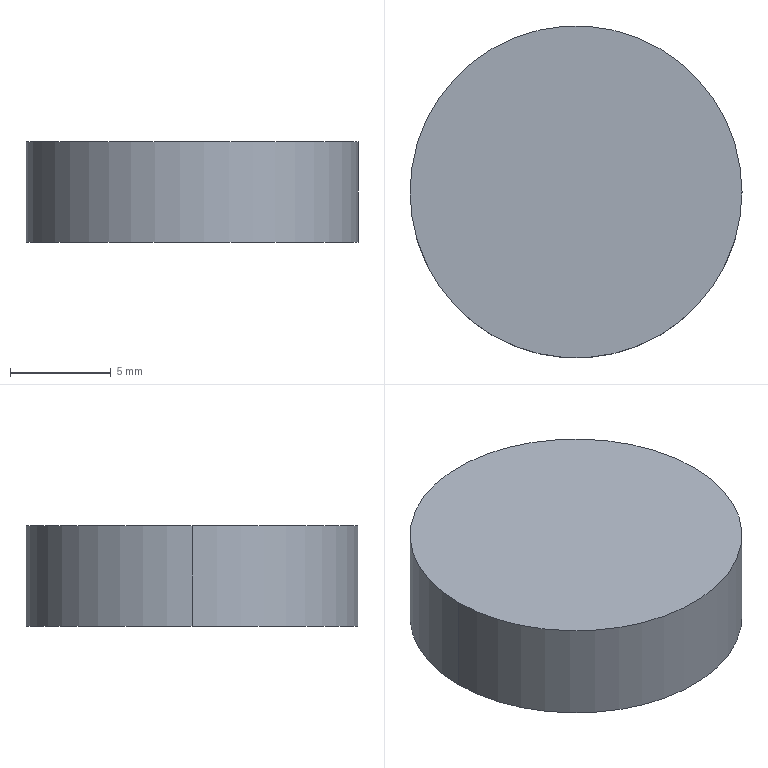Part | STEP file | Buzzer | 1 solid | 4 faces | box 16.5 x 16.5 x 5 mm | volume 1069 mm3 | cylinder 2 | plane 2 | commonest cylinder face diameters 16.5 x2
STEP:
#1=CARTESIAN_POINT('',(0.,0.,0.));
#2=DIRECTION('',(0.,0.,1.));
#3=DIRECTION('',(1.,0.,0.));
#4=AXIS2_PLACEMENT_3D('',#1,#2,#3);
#5=CARTESIAN_POINT('',(8.25,0.,5.));
#6=VERTEX_POINT('',#5);
#7=CARTESIAN_POINT('',(-8.25,0.,5.));
#8=VERTEX_POINT('',#7);
#9=CARTESIAN_POINT('',(0.,0.,5.));
#10=DIRECTION('',(0.,0.,1.));
#11=DIRECTION('',(-1.,0.,0.));
#12=AXIS2_PLACEMENT_3D('',#9,#10,#11);
#13=CIRCLE('',#12,8.25);
#14=CARTESIAN_POINT('',(0.,0.,5.));
#15=DIRECTION('',(0.,0.,-1.));
#16=DIRECTION('',(-1.,0.,0.));
#17=AXIS2_PLACEMENT_3D('',#14,#15,#16);
#18=CYLINDRICAL_SURFACE('',#17,8.25);
#19=CARTESIAN_POINT('',(6.283,0.));
#20=DIRECTION('',(-1.,0.));
#21=VECTOR('',#20,1.);
#22=LINE('',#19,#21);
#23=(GEOMETRIC_REPRESENTATION_CONTEXT(2)PARAMETRIC_REPRESENTATION_CONTEXT()REPRESENTATION_CONTEXT('',''));
#24=DEFINITIONAL_REPRESENTATION('',(#22),#23);
#25=PCURVE('',#18,#24);
#26=CARTESIAN_POINT('',(0.,0.,5.));
#27=DIRECTION('',(0.,0.,1.));
#28=DIRECTION('',(1.,0.,0.));
#29=AXIS2_PLACEMENT_3D('',#26,#27,#28);
#30=PLANE('',#29);
#31=CARTESIAN_POINT('',(0.,0.));
#32=DIRECTION('',(-1.,0.));
#33=AXIS2_PLACEMENT_2D('',#31,#32);
#34=CIRCLE('',#33,8.25);
#35=(GEOMETRIC_REPRESENTATION_CONTEXT(2)PARAMETRIC_REPRESENTATION_CONTEXT()REPRESENTATION_CONTEXT('',''));
#36=DEFINITIONAL_REPRESENTATION('',(#34),#35);
#37=PCURVE('',#30,#36);
#38=SURFACE_CURVE('',#13,(#25,#37),.PCURVE_S1.);
#39=EDGE_CURVE('',#6,#8,#38,.T.);
#40=ORIENTED_EDGE('',*,*,#39,.F.);
#41=CARTESIAN_POINT('',(8.25,0.,0.));
#42=VERTEX_POINT('',#41);
#43=CARTESIAN_POINT('',(8.25,0.,5.));
#44=DIRECTION('',(0.,0.,-1.));
#45=VECTOR('',#44,1.);
#46=LINE('',#43,#45);
#47=CARTESIAN_POINT('',(3.142,0.));
#48=DIRECTION('',(0.,1.));
#49=VECTOR('',#48,1.);
#50=LINE('',#47,#49);
#51=(GEOMETRIC_REPRESENTATION_CONTEXT(2)PARAMETRIC_REPRESENTATION_CONTEXT()REPRESENTATION_CONTEXT('',''));
#52=DEFINITIONAL_REPRESENTATION('',(#50),#51);
#53=PCURVE('',#18,#52);
#54=CARTESIAN_POINT('',(0.,0.,5.));
#55=DIRECTION('',(0.,0.,-1.));
#56=DIRECTION('',(-1.,0.,0.));
#57=AXIS2_PLACEMENT_3D('',#54,#55,#56);
#58=CYLINDRICAL_SURFACE('',#57,8.25);
#59=CARTESIAN_POINT('',(3.142,0.));
#60=DIRECTION('',(0.,1.));
#61=VECTOR('',#60,1.);
#62=LINE('',#59,#61);
#63=(GEOMETRIC_REPRESENTATION_CONTEXT(2)PARAMETRIC_REPRESENTATION_CONTEXT()REPRESENTATION_CONTEXT('',''));
#64=DEFINITIONAL_REPRESENTATION('',(#62),#63);
#65=PCURVE('',#58,#64);
#66=SURFACE_CURVE('',#46,(#53,#65),.PCURVE_S1.);
#67=EDGE_CURVE('',#6,#42,#66,.T.);
#68=ORIENTED_EDGE('',*,*,#67,.T.);
#69=CARTESIAN_POINT('',(-8.25,0.,0.));
#70=VERTEX_POINT('',#69);
#71=CARTESIAN_POINT('',(0.,0.,0.));
#72=DIRECTION('',(0.,0.,1.));
#73=DIRECTION('',(-1.,0.,0.));
#74=AXIS2_PLACEMENT_3D('',#71,#72,#73);
#75=CIRCLE('',#74,8.25);
#76=CARTESIAN_POINT('',(6.283,5.));
#77=DIRECTION('',(-1.,0.));
#78=VECTOR('',#77,1.);
#79=LINE('',#76,#78);
#80=(GEOMETRIC_REPRESENTATION_CONTEXT(2)PARAMETRIC_REPRESENTATION_CONTEXT()REPRESENTATION_CONTEXT('',''));
#81=DEFINITIONAL_REPRESENTATION('',(#79),#80);
#82=PCURVE('',#18,#81);
#83=CARTESIAN_POINT('',(0.,0.,0.));
#84=DIRECTION('',(0.,0.,1.));
#85=DIRECTION('',(1.,0.,0.));
#86=AXIS2_PLACEMENT_3D('',#83,#84,#85);
#87=PLANE('',#86);
#88=CARTESIAN_POINT('',(0.,0.));
#89=DIRECTION('',(-1.,0.));
#90=AXIS2_PLACEMENT_2D('',#88,#89);
#91=CIRCLE('',#90,8.25);
#92=(GEOMETRIC_REPRESENTATION_CONTEXT(2)PARAMETRIC_REPRESENTATION_CONTEXT()REPRESENTATION_CONTEXT('',''));
#93=DEFINITIONAL_REPRESENTATION('',(#91),#92);
#94=PCURVE('',#87,#93);
#95=SURFACE_CURVE('',#75,(#82,#94),.PCURVE_S1.);
#96=EDGE_CURVE('',#42,#70,#95,.T.);
#97=ORIENTED_EDGE('',*,*,#96,.T.);
#98=CARTESIAN_POINT('',(-8.25,0.,5.));
#99=DIRECTION('',(0.,0.,-1.));
#100=VECTOR('',#99,1.);
#101=LINE('',#98,#100);
#102=CARTESIAN_POINT('',(0.,0.));
#103=DIRECTION('',(0.,1.));
#104=VECTOR('',#103,1.);
#105=LINE('',#102,#104);
#106=(GEOMETRIC_REPRESENTATION_CONTEXT(2)PARAMETRIC_REPRESENTATION_CONTEXT()REPRESENTATION_CONTEXT('',''));
#107=DEFINITIONAL_REPRESENTATION('',(#105),#106);
#108=PCURVE('',#18,#107);
#109=CARTESIAN_POINT('',(6.283,0.));
#110=DIRECTION('',(0.,1.));
#111=VECTOR('',#110,1.);
#112=LINE('',#109,#111);
#113=(GEOMETRIC_REPRESENTATION_CONTEXT(2)PARAMETRIC_REPRESENTATION_CONTEXT()REPRESENTATION_CONTEXT('',''));
#114=DEFINITIONAL_REPRESENTATION('',(#112),#113);
#115=PCURVE('',#58,#114);
#116=SURFACE_CURVE('',#101,(#108,#115),.PCURVE_S1.);
#117=EDGE_CURVE('',#8,#70,#116,.T.);
#118=ORIENTED_EDGE('',*,*,#117,.F.);
#119=EDGE_LOOP('',(#40,#68,#97,#118));
#120=FACE_BOUND('',#119,.T.);
#121=ADVANCED_FACE('',(#120),#18,.T.);
#122=CARTESIAN_POINT('',(0.,0.,5.));
#123=DIRECTION('',(0.,0.,1.));
#124=DIRECTION('',(-1.,0.,0.));
#125=AXIS2_PLACEMENT_3D('',#122,#123,#124);
#126=CIRCLE('',#125,8.25);
#127=CARTESIAN_POINT('',(0.,0.));
#128=DIRECTION('',(-1.,0.));
#129=AXIS2_PLACEMENT_2D('',#127,#128);
#130=CIRCLE('',#129,8.25);
#131=(GEOMETRIC_REPRESENTATION_CONTEXT(2)PARAMETRIC_REPRESENTATION_CONTEXT()REPRESENTATION_CONTEXT('',''));
#132=DEFINITIONAL_REPRESENTATION('',(#130),#131);
#133=PCURVE('',#30,#132);
#134=CARTESIAN_POINT('',(6.283,0.));
#135=DIRECTION('',(-1.,0.));
#136=VECTOR('',#135,1.);
#137=LINE('',#134,#136);
#138=(GEOMETRIC_REPRESENTATION_CONTEXT(2)PARAMETRIC_REPRESENTATION_CONTEXT()REPRESENTATION_CONTEXT('',''));
#139=DEFINITIONAL_REPRESENTATION('',(#137),#138);
#140=PCURVE('',#58,#139);
#141=SURFACE_CURVE('',#126,(#133,#140),.PCURVE_S1.);
#142=EDGE_CURVE('',#8,#6,#141,.T.);
#143=ORIENTED_EDGE('',*,*,#142,.T.);
#144=ORIENTED_EDGE('',*,*,#39,.T.);
#145=EDGE_LOOP('',(#143,#144));
#146=FACE_BOUND('',#145,.T.);
#147=ADVANCED_FACE('',(#146),#30,.T.);
#148=ORIENTED_EDGE('',*,*,#67,.F.);
#149=ORIENTED_EDGE('',*,*,#142,.F.);
#150=ORIENTED_EDGE('',*,*,#117,.T.);
#151=CARTESIAN_POINT('',(0.,0.,0.));
#152=DIRECTION('',(0.,0.,1.));
#153=DIRECTION('',(-1.,0.,0.));
#154=AXIS2_PLACEMENT_3D('',#151,#152,#153);
#155=CIRCLE('',#154,8.25);
#156=CARTESIAN_POINT('',(6.283,5.));
#157=DIRECTION('',(-1.,0.));
#158=VECTOR('',#157,1.);
#159=LINE('',#156,#158);
#160=(GEOMETRIC_REPRESENTATION_CONTEXT(2)PARAMETRIC_REPRESENTATION_CONTEXT()REPRESENTATION_CONTEXT('',''));
#161=DEFINITIONAL_REPRESENTATION('',(#159),#160);
#162=PCURVE('',#58,#161);
#163=CARTESIAN_POINT('',(0.,0.));
#164=DIRECTION('',(-1.,0.));
#165=AXIS2_PLACEMENT_2D('',#163,#164);
#166=CIRCLE('',#165,8.25);
#167=(GEOMETRIC_REPRESENTATION_CONTEXT(2)PARAMETRIC_REPRESENTATION_CONTEXT()REPRESENTATION_CONTEXT('',''));
#168=DEFINITIONAL_REPRESENTATION('',(#166),#167);
#169=PCURVE('',#87,#168);
#170=SURFACE_CURVE('',#155,(#162,#169),.PCURVE_S1.);
#171=EDGE_CURVE('',#70,#42,#170,.T.);
#172=ORIENTED_EDGE('',*,*,#171,.T.);
#173=EDGE_LOOP('',(#148,#149,#150,#172));
#174=FACE_BOUND('',#173,.T.);
#175=ADVANCED_FACE('',(#174),#58,.T.);
#176=ORIENTED_EDGE('',*,*,#171,.F.);
#177=ORIENTED_EDGE('',*,*,#96,.F.);
#178=EDGE_LOOP('',(#176,#177));
#179=FACE_BOUND('',#178,.T.);
#180=ADVANCED_FACE('',(#179),#87,.F.);
#181=CLOSED_SHELL('',(#121,#147,#175,#180));
#182=MANIFOLD_SOLID_BREP('',#181);
#183=(LENGTH_UNIT()NAMED_UNIT(*)SI_UNIT(.MILLI.,.METRE.));
#184=UNCERTAINTY_MEASURE_WITH_UNIT(LENGTH_MEASURE(0.0000001),#183,'','');
#185=(NAMED_UNIT(*)PLANE_ANGLE_UNIT()SI_UNIT($,.RADIAN.));
#186=(NAMED_UNIT(*)SI_UNIT($,.STERADIAN.)SOLID_ANGLE_UNIT());
#187=(GEOMETRIC_REPRESENTATION_CONTEXT(3)GLOBAL_UNCERTAINTY_ASSIGNED_CONTEXT((#184))GLOBAL_UNIT_ASSIGNED_CONTEXT((#183,#185,#186))REPRESENTATION_CONTEXT('',''));
#188=ADVANCED_BREP_SHAPE_REPRESENTATION('',(#4,#182),#187);